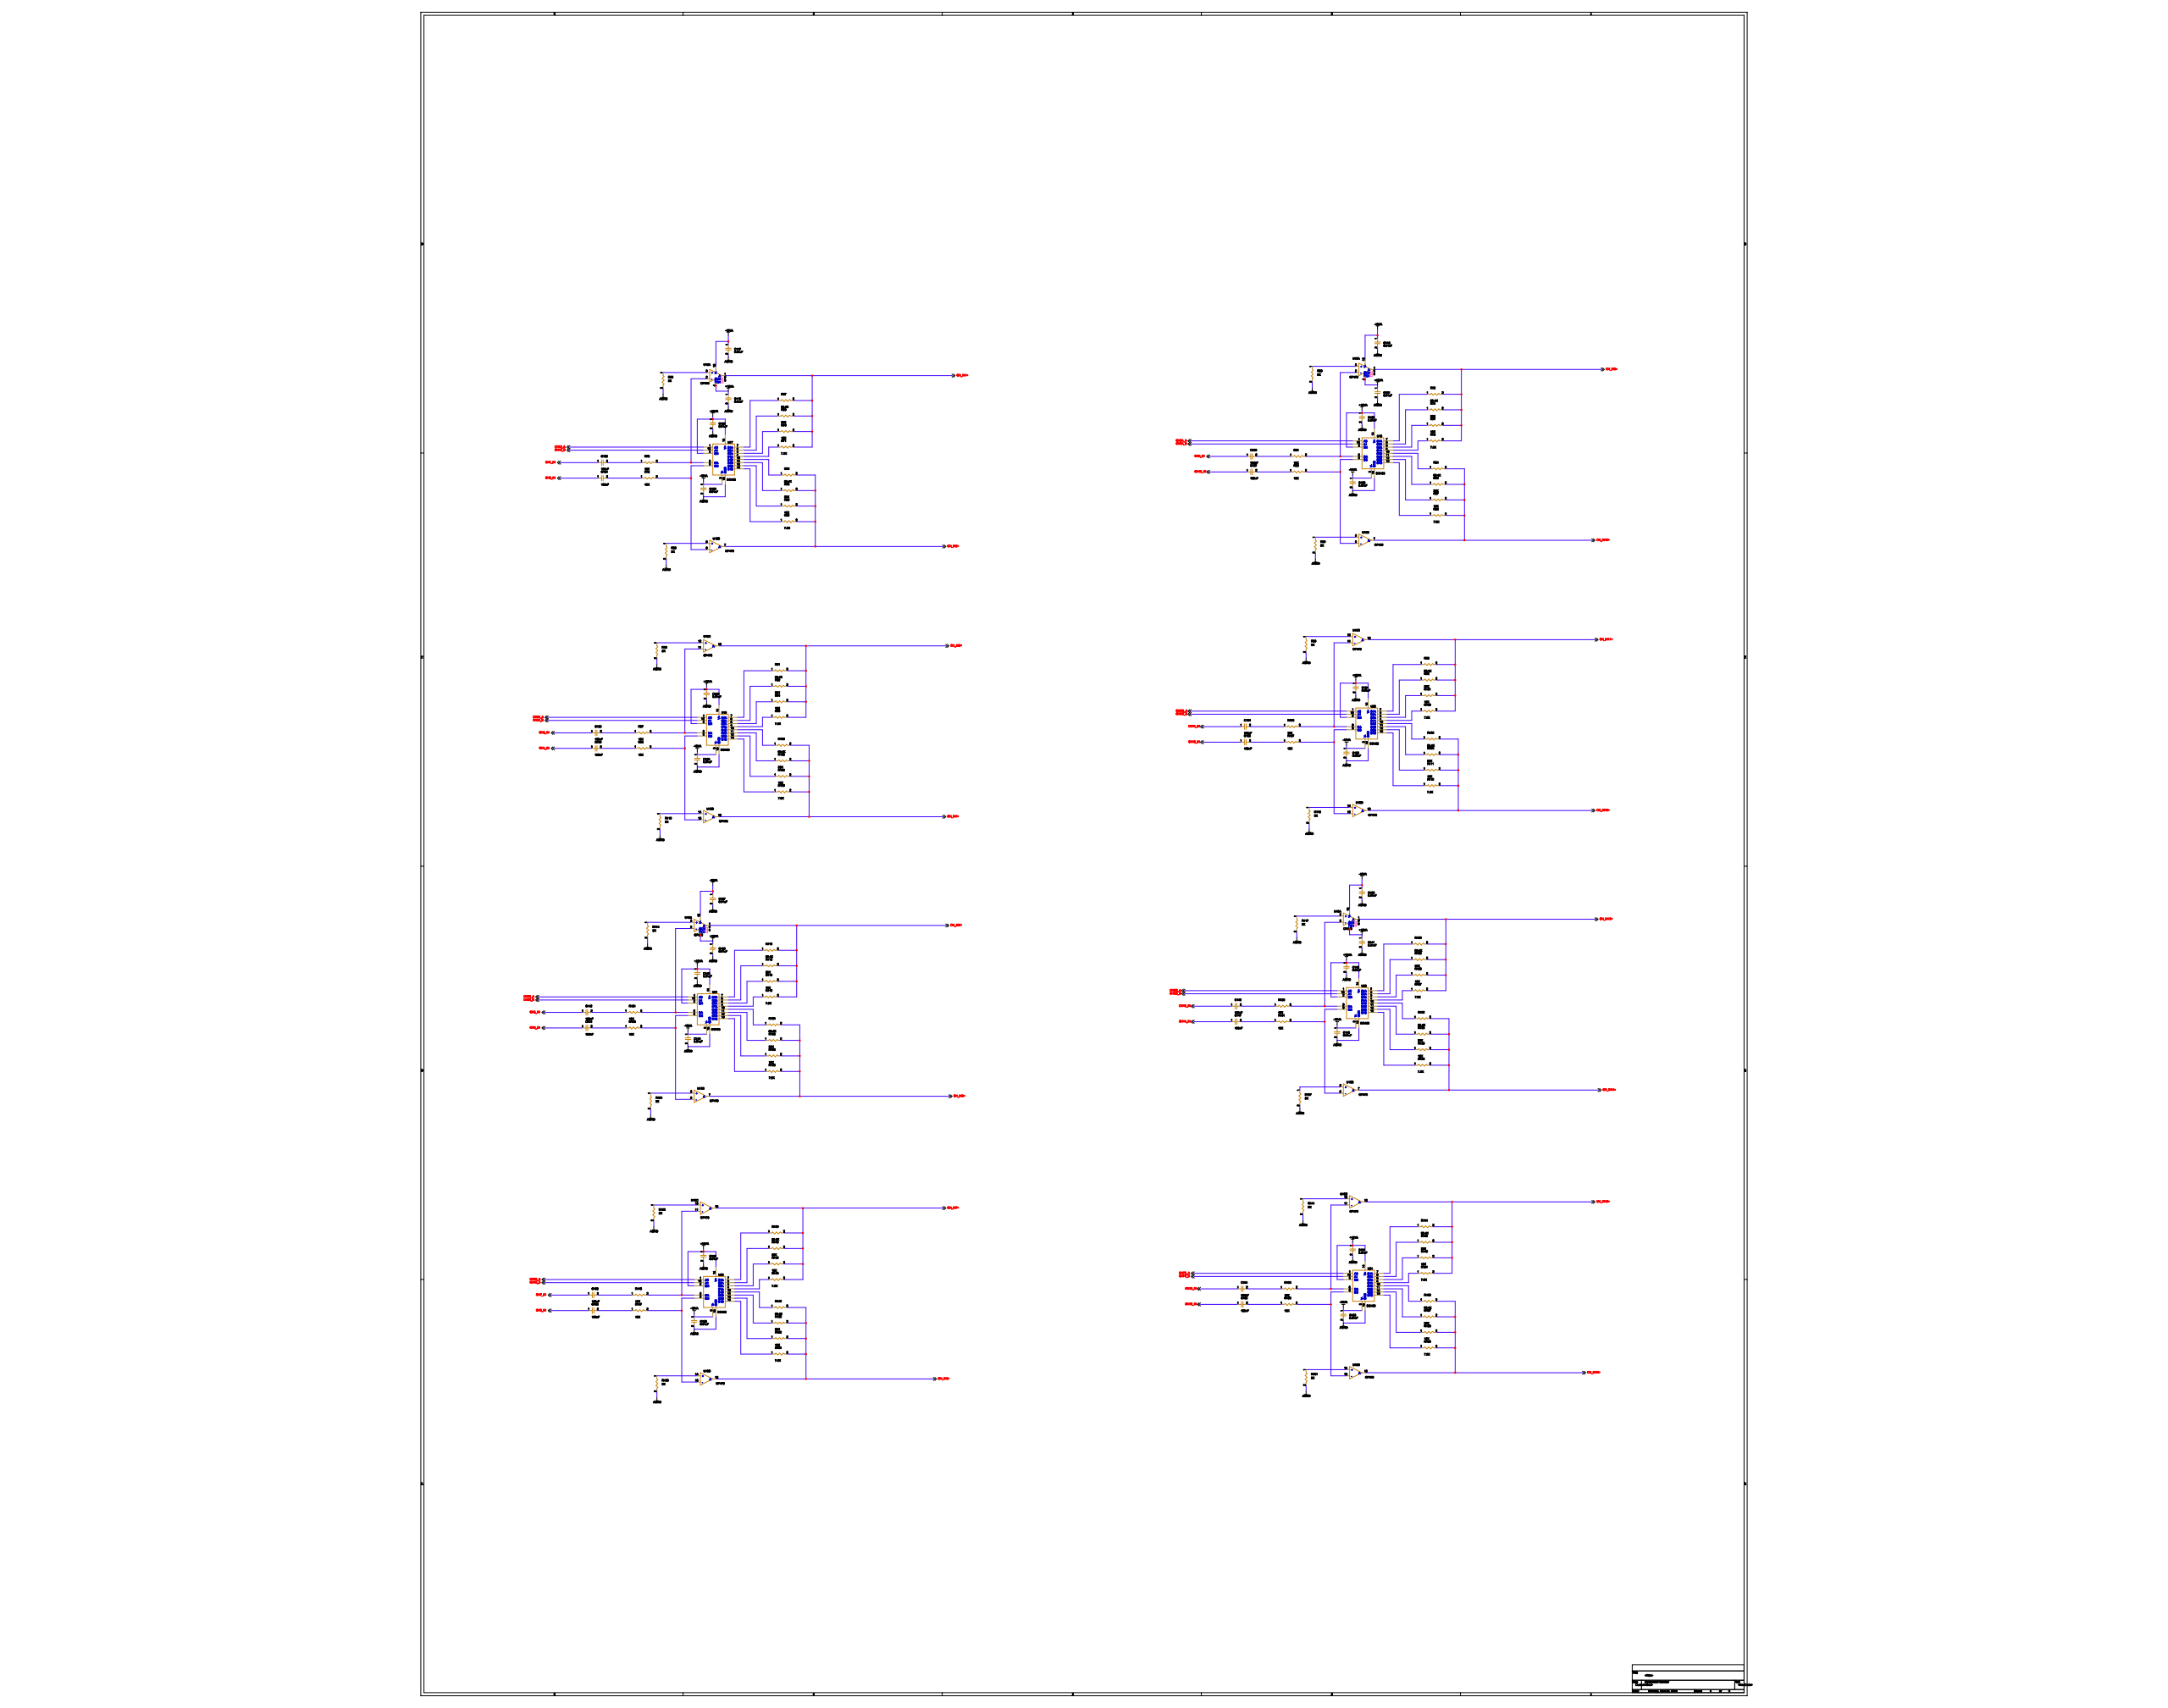Circuit board | Cadence Allegro | 362 parts | 391 nets | one sheet of the schematic
Parts on this sheet (reference | value | footprint):
C117 | 0.01uF | 1206
C118 | 0.01uF | 1206
C119 | 0.01uF | 1206
C120 | 0.01uF | 1206
C121 | 0.01uF | 1206
C122 | 100nF | 1206
C123 | 0.01uF | 1206
C124 | 100nF | 1206
C125 | 0.01uF | 1206
C126 | 100nF | 1206
C127 | 100nF | 1206
C128 | 0.01uF | 1206
C129 | 0.01uF | 1206
C130 | 100nF | 1206
C131 | 0.01uF | 1206
C132 | 100nF | 1206
C133 | 0.01uF | 1206
C134 | 100nF | 1206
C135 | 100nF | 1206
C136 | 0.01uF | 1206
C137 | 0.01uF | 1206
C138 | 0.01uF | 1206
C139 | 0.01uF | 1206
C140 | 0.01uF | 1206
C141 | 0.01uF | 1206
C142 | 100nF | 1206
C143 | 0.01uF | 1206
C144 | 100nF | 1206
C145 | 0.01uF | 1206
C146 | 100nF | 1206
C147 | 100nF | 1206
C148 | 0.01uF | 1206
C149 | 0.01uF | 1206
C150 | 100nF | 1206
C151 | 0.01uF | 1206
C152 | 100nF | 1206
C153 | 0.01uF | 1206
C154 | 100nF | 1206
C155 | 100nF | 1206
C156 | 0.01uF | 1206
R67 | 60.4K | 1206
R68 | 30K | 1206
R70 | 15K | 1206
R72 | 60.4K | 1206
R73 | 10K | 1206
R74 | 30K | 1206
R75 | 10K | 1206
R76 | 60.4K | 1206
R77 | 15K | 1206
R78 | 30K | 1206
R80 | 15K | 1206
R81 | 10K | 1206
R82 | 7.5K | 1206
R83 | 10K | 1206
R84 | 60.4K | 1206
R85 | 30K | 1206
R86 | 3K | 1206
R87 | 15K | 1206
R88 | 7.5K | 1206
R89 | 3K | 1206
R90 | 3K | 1206
R91 | 60.4K | 1206
R92 | 30K | 1206
R93 | 3K | 1206
R94 | 15K | 1206
R96 | 60.4K | 1206
R97 | 10K | 1206
R98 | 30K | 1206
R99 | 10K | 1206
R100 | 60.4K | 1206
R101 | 15K | 1206
R102 | 30K | 1206
R104 | 15K | 1206
R105 | 10K | 1206
R106 | 7.5K | 1206
R107 | 10K | 1206
R108 | 60.4K | 1206
R109 | 30K | 1206
R110 | 3K | 1206
R111 | 15K | 1206
R112 | 7.5K | 1206
R113 | 3K | 1206
R115 | 60.4K | 1206
R116 | 30K | 1206
R118 | 15K | 1206
R120 | 60.4K | 1206
R121 | 10K | 1206
R122 | 30K | 1206
R123 | 10K | 1206
R124 | 60.4K | 1206
R125 | 15K | 1206
R126 | 30K | 1206
R128 | 15K | 1206
R129 | 10K | 1206
R130 | 7.5K | 1206
R131 | 10K | 1206
R132 | 60.4K | 1206
R133 | 30K | 1206
R134 | 3K | 1206
R135 | 15K | 1206
R136 | 7.5K | 1206
R137 | 3K | 1206
R138 | 3K | 1206
R139 | 60.4K | 1206
R140 | 30K | 1206
R141 | 3K | 1206
R142 | 15K | 1206
R144 | 60.4K | 1206
R145 | 10K | 1206
R146 | 30K | 1206
R147 | 10K | 1206
R148 | 60.4K | 1206
R149 | 15K | 1206
R150 | 30K | 1206
R152 | 15K | 1206
R153 | 10K | 1206
R154 | 7.5K | 1206
R155 | 10K | 1206
R156 | 60.4K | 1206
R157 | 30K | 1206
R158 | 3K | 1206
R159 | 15K | 1206
R160 | 7.5K | 1206
R161 | 3K | 1206
U17 | DG406 | SO-16
U18 | DG406 | SO-16
U19 | DG406 | SO-16
U20 | DG406 | SO-16
U21 | DG406 | SO-16
U22 | DG406 | SO-16
U23 | DG406 | SO-16
U24 | DG406 | SO-16
Nets of these parts (net: part-pin ...):
+12VA: C119-1 C120-1 C121-1 C123-1 C129-1 C131-1 C139-1 C140-1 C141-1 C143-1 C149-1 C151-1 U17-2 U17-14 U18-2 U18-14 U19-2 U19-14 U20-2 U20-14 U21-2 U21-14 U22-2 U22-14 U23-2 U23-14 U24-2 U24-14
-12VA: C117-1 C118-1 C125-1 C128-1 C133-1 C136-1 C137-1 C138-1 C145-1 C148-1 C153-1 C156-1 U17-3 U18-3 U19-3 U20-3 U21-3 U22-3 U23-3 U24-3
AGND: C117-2 C118-2 C119-2 C120-2 C121-2 C123-2 C125-2 C128-2 C129-2 C131-2 C133-2 C136-2 C137-2 C138-2 C139-2 C140-2 C141-2 C143-2 C145-2 C148-2 C149-2 C151-2 C153-2 C156-2 R86-2 R89-2 R90-2 R93-2 R110-2 R113-2 R134-2 R137-2 R138-2 R141-2 R158-2 R161-2 U17-15 U18-15 U19-15 U20-15 U21-15 U22-15 U23-15 U24-15
N17391931: R129-2 U22-8
CH_IN13+: R120-2 R122-2 R125-2
N17392208: R137-1
N17392105: R131-2 U22-9
CH_IN14+: R132-2 R133-2 R135-2 R136-2
N17392243: R141-1
N17392263: R153-2 U24-8
CH_IN15+: R144-2 R146-2 R149-2
N17392514: R161-1
N17392411: R155-2 U24-9
CH_IN16+: R156-2 R157-2 R159-2 R160-2
N17391243: R81-2 U18-8
CH_IN9+: R72-2 R74-2 R77-2
N17391540: R89-1
N17391425: R83-2 U18-9
CH_IN10+: R84-2 R85-2 R87-2 R88-2
N17391575: R93-1
N17391595: R105-2 U20-8
CH_IN11+: R96-2 R98-2 R101-2
N17391846: R113-1
N17391743: R107-2 U20-9
CH_IN12+: R108-2 R109-2 R111-2 R112-2
N17386885: R121-2 U21-8
CH_IN5+: R115-2 R116-2 R118-2
N17387160: R134-1
N17387057: R123-2 U21-9
CH_IN6+: R124-2 R126-2 R128-2 R130-2
N17388522: R138-1
N17388538: R145-2 U23-8
CH_IN7+: R139-2 R140-2 R142-2
N17388815: R158-1
N17388712: R147-2 U23-9
CH_IN8+: R148-2 R150-2 R152-2 R154-2
N17386173: R73-2 U17-8
CH_IN1+: R67-2 R68-2 R70-2
N17386450: R86-1
N17386347: R75-2 U17-9
CH_IN2+: R76-2 R78-2 R80-2 R82-2
N17386519: R90-1
N17386535: R97-2 U19-8
CH_IN3+: R91-2 R92-2 R94-2
N17386812: R110-1
N17386709: R99-2 U19-9
CH_IN4+: R100-2 R102-2 R104-2 R106-2
CHF0_A: U24-1
CHF0_B: U24-16
N17392383: U24-4
N17392419: R160-1 U24-13
N17392341: R149-1 U24-5
N17392415: R159-1 U24-12
N17392303: R146-1 U24-6
N17392407: R157-1 U24-11
N17392281: R144-1 U24-7
N17392399: R156-1 U24-10
CH78_A: U23-1
CH78_B: U23-16
N17388684: U23-4
N17388720: R154-1 U23-13
N17388642: R142-1 U23-5
N17388716: R152-1 U23-12
N17388604: R140-1 U23-6
N17388708: R150-1 U23-11
N17388576: R139-1 U23-7
N17388700: R148-1 U23-10
CHDE_A: U22-1
CHDE_B: U22-16
N17392077: U22-4
N17392113: R136-1 U22-13
N17392035: R125-1 U22-5
N17392109: R135-1 U22-12
N17391997: R122-1 U22-6
N17392101: R133-1 U22-11
N17391969: R120-1 U22-7
N17392093: R132-1 U22-10
CH56_A: U21-1
CH56_B: U21-16
N17387029: U21-4
N17387065: R130-1 U21-13
N17386987: R118-1 U21-5
N17387061: R128-1 U21-12
N17386949: R116-1 U21-6
N17387053: R126-1 U21-11
N17386921: R115-1 U21-7
N17387045: R124-1 U21-10
CHBC_A: U20-1
CHBC_B: U20-16
N17391715: U20-4
N17391751: R112-1 U20-13
N17391673: R101-1 U20-5
N17391747: R111-1 U20-12
N17391635: R98-1 U20-6
N17391739: R109-1 U20-11
N17391613: R96-1 U20-7
N17391731: R108-1 U20-10
CH34_A: U19-1
CH34_B: U19-16
N17386681: U19-4
N17386717: R106-1 U19-13
N17386639: R94-1 U19-5
N17386713: R104-1 U19-12
N17386601: R92-1 U19-6
N17386705: R102-1 U19-11
N17386573: R91-1 U19-7
N17386697: R100-1 U19-10
CH9A_A: U18-1
CH9A_B: U18-16
N17391389: U18-4
N17391433: R88-1 U18-13
N17391347: R77-1 U18-5
N17391429: R87-1 U18-12
N17391309: R74-1 U18-6
N17391421: R85-1 U18-11
N17391281: R72-1 U18-7
N17391413: R84-1 U18-10
CH12_A: U17-1
CH12_B: U17-16
N17386319: U17-4
N17386355: R82-1 U17-13
N17386277: R70-1 U17-5
N17386351: R80-1 U17-12
N17386239: R68-1 U17-6
N17386343: R78-1 U17-11
N17386211: R67-1 U17-7
N17386335: R76-1 U17-10
CH16_IN: C155-1
CH15_IN: C154-1
CH1_IN: C122-1
CH2_IN: C124-1
CH3_IN: C130-1
CH4_IN: C132-1
CH5_IN: C142-1
CH6_IN: C144-1
CH7_IN: C150-1
CH8_IN: C152-1
CH9_IN: C126-1
CH10_IN: C127-1
CH11_IN: C134-1
CH12_IN: C135-1
CH13_IN: C146-1
CH14_IN: C147-1
N17394680: C155-2 R155-1
N17394654: C154-2 R153-1
N17394145: C152-2 R147-1
N17394119: C150-2 R145-1
N17394545: C147-2 R131-1
N17394519: C146-2 R129-1
N17394023: C144-2 R123-1
N17393997: C142-2 R121-1
N17394412: C135-2 R107-1
N17394386: C134-2 R105-1
N17393902: C132-2 R99-1
N17393876: C130-2 R97-1
N17394281: C127-2 R83-1
N17394255: C126-2 R81-1
N17393618: C124-2 R75-1
N17393615: C122-2 R73-1